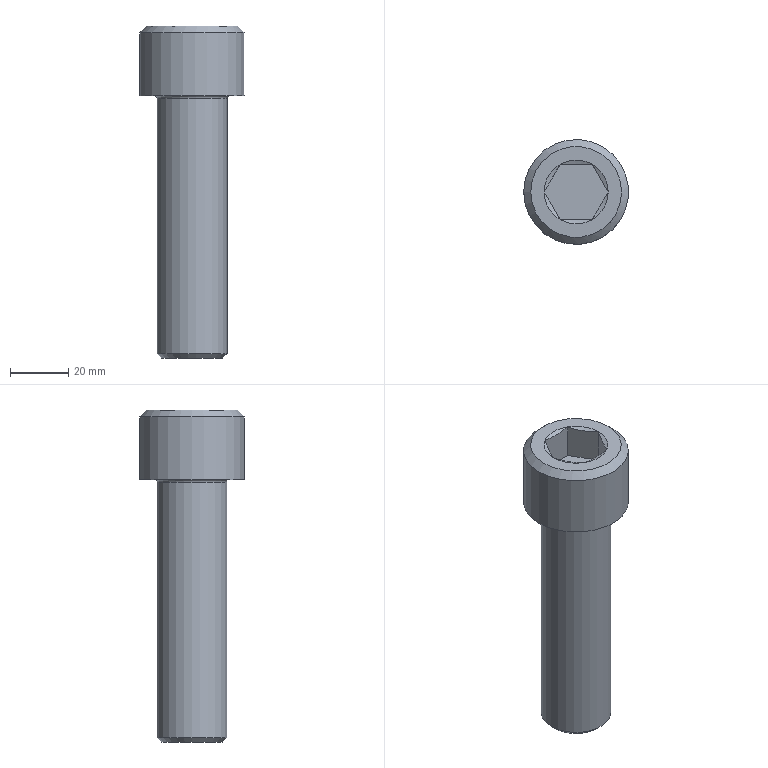Part | STEP file | solid 129 | 1 solid | 21 faces | box 36 x 36 x 114 mm | volume 60994 mm3 | plane 10 | sphere 6 | cylinder 2 | cone 2 | torus 1 | commonest cylinder face diameters 24 x1 36 x1